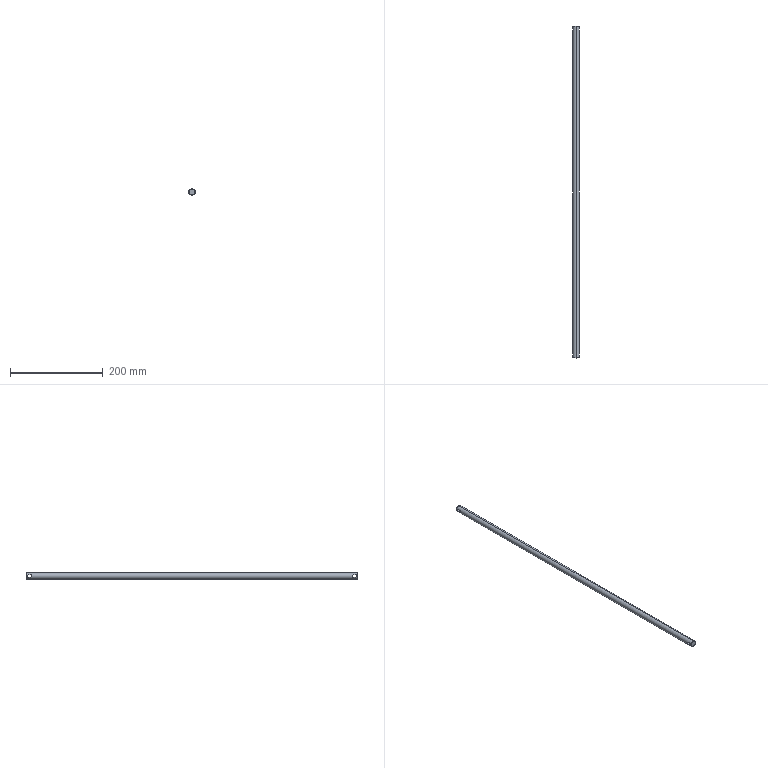Part | SolidWorks | features Chamfer 1, Extrusion 1, ICE 1 | 1 solid | 16 faces | box 14 x 715 x 14 mm | volume 108794 mm3 | cylinder 6 | plane 6 | cone 4 | commonest cylinder face diameters 6 x4 14 x2
STEP:
#1=CARTESIAN_POINT('',(0.,357.5,6.5));
#2=VERTEX_POINT('',#1);
#3=CARTESIAN_POINT('',(0.,357.5,-6.5));
#4=VERTEX_POINT('',#3);
#5=CARTESIAN_POINT('',(0.,357.5,0.));
#6=DIRECTION('',(0.,1.,0.));
#7=DIRECTION('',(0.,0.,1.));
#8=AXIS2_PLACEMENT_3D('',#5,#6,#7);
#9=CIRCLE('',#8,6.5);
#10=EDGE_CURVE('',#2,#4,#9,.T.);
#11=ORIENTED_EDGE('',*,*,#10,.F.);
#12=CARTESIAN_POINT('',(0.,357.,7.));
#13=VERTEX_POINT('',#12);
#14=CARTESIAN_POINT('',(0.,357.5,6.5));
#15=DIRECTION('',(0.,-0.7071,0.7071));
#16=VECTOR('',#15,1000.);
#17=LINE('',#14,#16);
#18=EDGE_CURVE('',#2,#13,#17,.T.);
#19=ORIENTED_EDGE('',*,*,#18,.T.);
#20=CARTESIAN_POINT('',(0.,357.,-7.));
#21=VERTEX_POINT('',#20);
#22=CARTESIAN_POINT('',(0.,357.,0.));
#23=DIRECTION('',(0.,-1.,0.));
#24=DIRECTION('',(0.,0.,1.));
#25=AXIS2_PLACEMENT_3D('',#22,#23,#24);
#26=CIRCLE('',#25,7.);
#27=EDGE_CURVE('',#21,#13,#26,.T.);
#28=ORIENTED_EDGE('',*,*,#27,.F.);
#29=CARTESIAN_POINT('',(0.,357.5,-6.5));
#30=DIRECTION('',(0.,-0.7071,-0.7071));
#31=VECTOR('',#30,1000.);
#32=LINE('',#29,#31);
#33=EDGE_CURVE('',#4,#21,#32,.T.);
#34=ORIENTED_EDGE('',*,*,#33,.F.);
#35=EDGE_LOOP('',(#11,#19,#28,#34));
#36=FACE_OUTER_BOUND('',#35,.T.);
#37=CARTESIAN_POINT('',(0.,357.5,0.));
#38=DIRECTION('',(0.,-1.,0.));
#39=DIRECTION('',(0.,0.,-1.));
#40=AXIS2_PLACEMENT_3D('',#37,#38,#39);
#41=CONICAL_SURFACE('',#40,6.5,0.7854);
#42=ADVANCED_FACE('',(#36),#41,.T.);
#43=CARTESIAN_POINT('',(0.,-357.5,-6.5));
#44=VERTEX_POINT('',#43);
#45=CARTESIAN_POINT('',(0.,-357.5,6.5));
#46=VERTEX_POINT('',#45);
#47=CARTESIAN_POINT('',(0.,-357.5,0.));
#48=DIRECTION('',(0.,-1.,0.));
#49=DIRECTION('',(0.,0.,1.));
#50=AXIS2_PLACEMENT_3D('',#47,#48,#49);
#51=CIRCLE('',#50,6.5);
#52=EDGE_CURVE('',#44,#46,#51,.T.);
#53=ORIENTED_EDGE('',*,*,#52,.F.);
#54=CARTESIAN_POINT('',(0.,-357.,-7.));
#55=VERTEX_POINT('',#54);
#56=CARTESIAN_POINT('',(0.,-357.,-7.));
#57=DIRECTION('',(0.,0.7071,-0.7071));
#58=VECTOR('',#57,1000.);
#59=LINE('',#56,#58);
#60=EDGE_CURVE('',#44,#55,#59,.T.);
#61=ORIENTED_EDGE('',*,*,#60,.T.);
#62=CARTESIAN_POINT('',(0.,-357.,7.));
#63=VERTEX_POINT('',#62);
#64=CARTESIAN_POINT('',(0.,-357.,0.));
#65=DIRECTION('',(0.,1.,0.));
#66=DIRECTION('',(0.,0.,1.));
#67=AXIS2_PLACEMENT_3D('',#64,#65,#66);
#68=CIRCLE('',#67,7.);
#69=EDGE_CURVE('',#63,#55,#68,.T.);
#70=ORIENTED_EDGE('',*,*,#69,.F.);
#71=CARTESIAN_POINT('',(0.,-357.,7.));
#72=DIRECTION('',(0.,0.7071,0.7071));
#73=VECTOR('',#72,1000.);
#74=LINE('',#71,#73);
#75=EDGE_CURVE('',#46,#63,#74,.T.);
#76=ORIENTED_EDGE('',*,*,#75,.F.);
#77=EDGE_LOOP('',(#53,#61,#70,#76));
#78=FACE_OUTER_BOUND('',#77,.T.);
#79=CARTESIAN_POINT('',(0.,-357.,0.));
#80=DIRECTION('',(0.,1.,0.));
#81=DIRECTION('',(0.,0.,1.));
#82=AXIS2_PLACEMENT_3D('',#79,#80,#81);
#83=CONICAL_SURFACE('',#82,7.,0.7854);
#84=ADVANCED_FACE('',(#78),#83,.T.);
#85=CARTESIAN_POINT('',(6.325,351.5,-3.));
#86=VERTEX_POINT('',#85);
#87=CARTESIAN_POINT('',(6.325,348.5,-3.));
#88=VERTEX_POINT('',#87);
#89=CARTESIAN_POINT('',(6.325,357.5,-3.));
#90=DIRECTION('',(0.,-1.,0.));
#91=VECTOR('',#90,1000.);
#92=LINE('',#89,#91);
#93=EDGE_CURVE('',#86,#88,#92,.T.);
#94=ORIENTED_EDGE('',*,*,#93,.T.);
#95=CARTESIAN_POINT('',(6.325,348.5,3.));
#96=VERTEX_POINT('',#95);
#97=CARTESIAN_POINT('',(6.325,348.5,-3.));
#98=CARTESIAN_POINT('',(6.325,348.299,-3.));
#99=CARTESIAN_POINT('',(6.334,348.102,-2.98));
#100=CARTESIAN_POINT('',(6.37,347.716,-2.902));
#101=CARTESIAN_POINT('',(6.397,347.524,-2.844));
#102=CARTESIAN_POINT('',(6.462,347.162,-2.692));
#103=CARTESIAN_POINT('',(6.5,346.991,-2.6));
#104=CARTESIAN_POINT('',(6.583,346.667,-2.383));
#105=CARTESIAN_POINT('',(6.627,346.515,-2.258));
#106=CARTESIAN_POINT('',(6.714,346.242,-1.985));
#107=CARTESIAN_POINT('',(6.757,346.118,-1.834));
#108=CARTESIAN_POINT('',(6.838,345.9,-1.509));
#109=CARTESIAN_POINT('',(6.873,345.808,-1.337));
#110=CARTESIAN_POINT('',(6.934,345.657,-0.977));
#111=CARTESIAN_POINT('',(6.959,345.598,-0.7853));
#112=CARTESIAN_POINT('',(6.991,345.52,-0.3967));
#113=CARTESIAN_POINT('',(7.,345.5,-0.2002));
#114=CARTESIAN_POINT('',(7.,345.5,0.197));
#115=CARTESIAN_POINT('',(6.991,345.52,0.3982));
#116=CARTESIAN_POINT('',(6.959,345.598,0.7855));
#117=CARTESIAN_POINT('',(6.934,345.656,0.9747));
#118=CARTESIAN_POINT('',(6.873,345.809,1.34));
#119=CARTESIAN_POINT('',(6.837,345.901,1.512));
#120=CARTESIAN_POINT('',(6.757,346.118,1.835));
#121=CARTESIAN_POINT('',(6.714,346.244,1.987));
#122=CARTESIAN_POINT('',(6.626,346.518,2.261));
#123=CARTESIAN_POINT('',(6.583,346.668,2.383));
#124=CARTESIAN_POINT('',(6.5,346.991,2.6));
#125=CARTESIAN_POINT('',(6.461,347.165,2.694));
#126=CARTESIAN_POINT('',(6.397,347.525,2.844));
#127=CARTESIAN_POINT('',(6.37,347.713,2.902));
#128=CARTESIAN_POINT('',(6.334,348.105,2.981));
#129=CARTESIAN_POINT('',(6.325,348.302,3.));
#130=CARTESIAN_POINT('',(6.325,348.5,3.));
#131=B_SPLINE_CURVE_WITH_KNOTS('',3,(#97,#98,#99,#100,#101,#102,#103,#104,#105,#106,#107,#108,#109,#110,#111,#112,#113,#114,#115,#116,#117,#118,#119,#120,#121,#122,#123,#124,#125,#126,#127,#128,#129,#130),.UNSPECIFIED.,.F.,.F.,(4,2,2,2,2,2,2,2,2,2,2,2,2,2,2,2,4),(0.,0.0005934,0.001187,0.00178,0.002374,0.002967,0.003561,0.004154,0.004748,0.005341,0.005934,0.006528,0.007121,0.007715,0.008308,0.008902,0.009495),.UNSPECIFIED.);
#132=EDGE_CURVE('',#88,#96,#131,.T.);
#133=ORIENTED_EDGE('',*,*,#132,.T.);
#134=CARTESIAN_POINT('',(6.325,351.5,3.));
#135=VERTEX_POINT('',#134);
#136=CARTESIAN_POINT('',(6.325,357.5,3.));
#137=DIRECTION('',(0.,1.,0.));
#138=VECTOR('',#137,1000.);
#139=LINE('',#136,#138);
#140=EDGE_CURVE('',#96,#135,#139,.T.);
#141=ORIENTED_EDGE('',*,*,#140,.T.);
#142=CARTESIAN_POINT('',(6.325,351.5,3.));
#143=CARTESIAN_POINT('',(6.325,351.698,3.));
#144=CARTESIAN_POINT('',(6.334,351.898,2.98));
#145=CARTESIAN_POINT('',(6.37,352.287,2.902));
#146=CARTESIAN_POINT('',(6.397,352.475,2.844));
#147=CARTESIAN_POINT('',(6.462,352.838,2.693));
#148=CARTESIAN_POINT('',(6.501,353.011,2.599));
#149=CARTESIAN_POINT('',(6.583,353.333,2.383));
#150=CARTESIAN_POINT('',(6.627,353.484,2.259));
#151=CARTESIAN_POINT('',(6.715,353.759,1.983));
#152=CARTESIAN_POINT('',(6.758,353.882,1.834));
#153=CARTESIAN_POINT('',(6.837,354.099,1.512));
#154=CARTESIAN_POINT('',(6.874,354.193,1.337));
#155=CARTESIAN_POINT('',(6.934,354.344,0.9749));
#156=CARTESIAN_POINT('',(6.958,354.402,0.7876));
#157=CARTESIAN_POINT('',(6.991,354.48,0.3996));
#158=CARTESIAN_POINT('',(7.,354.5,0.1985));
#159=CARTESIAN_POINT('',(7.,354.5,-0.1971));
#160=CARTESIAN_POINT('',(6.992,354.481,-0.3946));
#161=CARTESIAN_POINT('',(6.958,354.402,-0.7866));
#162=CARTESIAN_POINT('',(6.934,354.344,-0.9748));
#163=CARTESIAN_POINT('',(6.874,354.193,-1.337));
#164=CARTESIAN_POINT('',(6.837,354.099,-1.512));
#165=CARTESIAN_POINT('',(6.757,353.882,-1.835));
#166=CARTESIAN_POINT('',(6.714,353.759,-1.984));
#167=CARTESIAN_POINT('',(6.627,353.483,-2.26));
#168=CARTESIAN_POINT('',(6.583,353.332,-2.384));
#169=CARTESIAN_POINT('',(6.501,353.011,-2.599));
#170=CARTESIAN_POINT('',(6.462,352.838,-2.692));
#171=CARTESIAN_POINT('',(6.397,352.474,-2.844));
#172=CARTESIAN_POINT('',(6.37,352.286,-2.902));
#173=CARTESIAN_POINT('',(6.334,351.901,-2.98));
#174=CARTESIAN_POINT('',(6.325,351.701,-3.));
#175=CARTESIAN_POINT('',(6.325,351.5,-3.));
#176=B_SPLINE_CURVE_WITH_KNOTS('',3,(#142,#143,#144,#145,#146,#147,#148,#149,#150,#151,#152,#153,#154,#155,#156,#157,#158,#159,#160,#161,#162,#163,#164,#165,#166,#167,#168,#169,#170,#171,#172,#173,#174,#175),.UNSPECIFIED.,.F.,.F.,(4,2,2,2,2,2,2,2,2,2,2,2,2,2,2,2,4),(0.009495,0.01009,0.01068,0.01127,0.01187,0.01246,0.01305,0.01365,0.01424,0.01483,0.01542,0.01602,0.01661,0.0172,0.0178,0.01839,0.01898),.UNSPECIFIED.);
#177=EDGE_CURVE('',#135,#86,#176,.T.);
#178=ORIENTED_EDGE('',*,*,#177,.T.);
#179=EDGE_LOOP('',(#94,#133,#141,#178));
#180=FACE_BOUND('',#179,.T.);
#181=CARTESIAN_POINT('',(6.325,-351.5,3.));
#182=VERTEX_POINT('',#181);
#183=CARTESIAN_POINT('',(6.325,-348.5,3.));
#184=VERTEX_POINT('',#183);
#185=CARTESIAN_POINT('',(6.325,357.5,3.));
#186=DIRECTION('',(0.,1.,0.));
#187=VECTOR('',#186,1000.);
#188=LINE('',#185,#187);
#189=EDGE_CURVE('',#182,#184,#188,.T.);
#190=ORIENTED_EDGE('',*,*,#189,.T.);
#191=CARTESIAN_POINT('',(6.325,-348.5,-3.));
#192=VERTEX_POINT('',#191);
#193=CARTESIAN_POINT('',(6.325,-348.5,3.));
#194=CARTESIAN_POINT('',(6.325,-348.302,3.));
#195=CARTESIAN_POINT('',(6.334,-348.102,2.98));
#196=CARTESIAN_POINT('',(6.37,-347.713,2.902));
#197=CARTESIAN_POINT('',(6.397,-347.525,2.844));
#198=CARTESIAN_POINT('',(6.462,-347.162,2.693));
#199=CARTESIAN_POINT('',(6.501,-346.989,2.599));
#200=CARTESIAN_POINT('',(6.583,-346.667,2.383));
#201=CARTESIAN_POINT('',(6.627,-346.516,2.259));
#202=CARTESIAN_POINT('',(6.715,-346.241,1.983));
#203=CARTESIAN_POINT('',(6.758,-346.118,1.834));
#204=CARTESIAN_POINT('',(6.837,-345.901,1.512));
#205=CARTESIAN_POINT('',(6.874,-345.807,1.337));
#206=CARTESIAN_POINT('',(6.934,-345.656,0.9749));
#207=CARTESIAN_POINT('',(6.958,-345.598,0.7876));
#208=CARTESIAN_POINT('',(6.991,-345.52,0.3996));
#209=CARTESIAN_POINT('',(7.,-345.5,0.1985));
#210=CARTESIAN_POINT('',(7.,-345.5,-0.1971));
#211=CARTESIAN_POINT('',(6.992,-345.519,-0.3946));
#212=CARTESIAN_POINT('',(6.958,-345.598,-0.7866));
#213=CARTESIAN_POINT('',(6.934,-345.656,-0.9748));
#214=CARTESIAN_POINT('',(6.874,-345.807,-1.337));
#215=CARTESIAN_POINT('',(6.837,-345.901,-1.512));
#216=CARTESIAN_POINT('',(6.757,-346.118,-1.835));
#217=CARTESIAN_POINT('',(6.714,-346.241,-1.984));
#218=CARTESIAN_POINT('',(6.627,-346.517,-2.26));
#219=CARTESIAN_POINT('',(6.583,-346.668,-2.384));
#220=CARTESIAN_POINT('',(6.501,-346.989,-2.599));
#221=CARTESIAN_POINT('',(6.462,-347.162,-2.692));
#222=CARTESIAN_POINT('',(6.397,-347.526,-2.844));
#223=CARTESIAN_POINT('',(6.37,-347.714,-2.902));
#224=CARTESIAN_POINT('',(6.334,-348.099,-2.98));
#225=CARTESIAN_POINT('',(6.325,-348.299,-3.));
#226=CARTESIAN_POINT('',(6.325,-348.5,-3.));
#227=B_SPLINE_CURVE_WITH_KNOTS('',3,(#193,#194,#195,#196,#197,#198,#199,#200,#201,#202,#203,#204,#205,#206,#207,#208,#209,#210,#211,#212,#213,#214,#215,#216,#217,#218,#219,#220,#221,#222,#223,#224,#225,#226),.UNSPECIFIED.,.F.,.F.,(4,2,2,2,2,2,2,2,2,2,2,2,2,2,2,2,4),(0.009495,0.01009,0.01068,0.01127,0.01187,0.01246,0.01305,0.01365,0.01424,0.01483,0.01542,0.01602,0.01661,0.0172,0.0178,0.01839,0.01898),.UNSPECIFIED.);
#228=EDGE_CURVE('',#184,#192,#227,.T.);
#229=ORIENTED_EDGE('',*,*,#228,.T.);
#230=CARTESIAN_POINT('',(6.325,-351.5,-3.));
#231=VERTEX_POINT('',#230);
#232=CARTESIAN_POINT('',(6.325,357.5,-3.));
#233=DIRECTION('',(0.,-1.,0.));
#234=VECTOR('',#233,1000.);
#235=LINE('',#232,#234);
#236=EDGE_CURVE('',#192,#231,#235,.T.);
#237=ORIENTED_EDGE('',*,*,#236,.T.);
#238=CARTESIAN_POINT('',(6.325,-351.5,-3.));
#239=CARTESIAN_POINT('',(6.325,-351.701,-3.));
#240=CARTESIAN_POINT('',(6.334,-351.898,-2.98));
#241=CARTESIAN_POINT('',(6.37,-352.284,-2.902));
#242=CARTESIAN_POINT('',(6.397,-352.476,-2.844));
#243=CARTESIAN_POINT('',(6.462,-352.838,-2.692));
#244=CARTESIAN_POINT('',(6.5,-353.009,-2.6));
#245=CARTESIAN_POINT('',(6.583,-353.333,-2.383));
#246=CARTESIAN_POINT('',(6.627,-353.485,-2.258));
#247=CARTESIAN_POINT('',(6.714,-353.758,-1.985));
#248=CARTESIAN_POINT('',(6.757,-353.882,-1.834));
#249=CARTESIAN_POINT('',(6.838,-354.1,-1.509));
#250=CARTESIAN_POINT('',(6.873,-354.192,-1.337));
#251=CARTESIAN_POINT('',(6.934,-354.343,-0.977));
#252=CARTESIAN_POINT('',(6.959,-354.402,-0.7853));
#253=CARTESIAN_POINT('',(6.991,-354.48,-0.3967));
#254=CARTESIAN_POINT('',(7.,-354.5,-0.2002));
#255=CARTESIAN_POINT('',(7.,-354.5,0.197));
#256=CARTESIAN_POINT('',(6.991,-354.48,0.3982));
#257=CARTESIAN_POINT('',(6.959,-354.402,0.7855));
#258=CARTESIAN_POINT('',(6.934,-354.344,0.9747));
#259=CARTESIAN_POINT('',(6.873,-354.191,1.34));
#260=CARTESIAN_POINT('',(6.837,-354.099,1.512));
#261=CARTESIAN_POINT('',(6.757,-353.882,1.835));
#262=CARTESIAN_POINT('',(6.714,-353.756,1.987));
#263=CARTESIAN_POINT('',(6.626,-353.482,2.261));
#264=CARTESIAN_POINT('',(6.583,-353.332,2.383));
#265=CARTESIAN_POINT('',(6.5,-353.009,2.6));
#266=CARTESIAN_POINT('',(6.461,-352.835,2.694));
#267=CARTESIAN_POINT('',(6.397,-352.475,2.844));
#268=CARTESIAN_POINT('',(6.37,-352.287,2.902));
#269=CARTESIAN_POINT('',(6.334,-351.895,2.981));
#270=CARTESIAN_POINT('',(6.325,-351.698,3.));
#271=CARTESIAN_POINT('',(6.325,-351.5,3.));
#272=B_SPLINE_CURVE_WITH_KNOTS('',3,(#238,#239,#240,#241,#242,#243,#244,#245,#246,#247,#248,#249,#250,#251,#252,#253,#254,#255,#256,#257,#258,#259,#260,#261,#262,#263,#264,#265,#266,#267,#268,#269,#270,#271),.UNSPECIFIED.,.F.,.F.,(4,2,2,2,2,2,2,2,2,2,2,2,2,2,2,2,4),(0.,0.0005934,0.001187,0.00178,0.002374,0.002967,0.003561,0.004154,0.004748,0.005341,0.005934,0.006528,0.007121,0.007715,0.008308,0.008902,0.009495),.UNSPECIFIED.);
#273=EDGE_CURVE('',#231,#182,#272,.T.);
#274=ORIENTED_EDGE('',*,*,#273,.T.);
#275=EDGE_LOOP('',(#190,#229,#237,#274));
#276=FACE_BOUND('',#275,.T.);
#277=ORIENTED_EDGE('',*,*,#27,.T.);
#278=CARTESIAN_POINT('',(0.,357.5,7.));
#279=DIRECTION('',(0.,-1.,0.));
#280=VECTOR('',#279,1000.);
#281=LINE('',#278,#280);
#282=EDGE_CURVE('',#13,#63,#281,.T.);
#283=ORIENTED_EDGE('',*,*,#282,.T.);
#284=ORIENTED_EDGE('',*,*,#69,.T.);
#285=CARTESIAN_POINT('',(0.,357.5,-7.));
#286=DIRECTION('',(0.,-1.,0.));
#287=VECTOR('',#286,1000.);
#288=LINE('',#285,#287);
#289=EDGE_CURVE('',#21,#55,#288,.T.);
#290=ORIENTED_EDGE('',*,*,#289,.F.);
#291=EDGE_LOOP('',(#277,#283,#284,#290));
#292=FACE_OUTER_BOUND('',#291,.T.);
#293=CARTESIAN_POINT('',(0.,357.5,0.));
#294=DIRECTION('',(0.,-1.,0.));
#295=DIRECTION('',(0.,0.,-1.));
#296=AXIS2_PLACEMENT_3D('',#293,#294,#295);
#297=CYLINDRICAL_SURFACE('',#296,7.);
#298=ADVANCED_FACE('',(#180,#276,#292),#297,.T.);
#299=ORIENTED_EDGE('',*,*,#282,.F.);
#300=CARTESIAN_POINT('',(0.,357.,0.));
#301=DIRECTION('',(0.,-1.,0.));
#302=DIRECTION('',(0.,0.,1.));
#303=AXIS2_PLACEMENT_3D('',#300,#301,#302);
#304=CIRCLE('',#303,7.);
#305=EDGE_CURVE('',#13,#21,#304,.T.);
#306=ORIENTED_EDGE('',*,*,#305,.T.);
#307=ORIENTED_EDGE('',*,*,#289,.T.);
#308=CARTESIAN_POINT('',(0.,-357.,0.));
#309=DIRECTION('',(0.,1.,0.));
#310=DIRECTION('',(0.,0.,1.));
#311=AXIS2_PLACEMENT_3D('',#308,#309,#310);
#312=CIRCLE('',#311,7.);
#313=EDGE_CURVE('',#55,#63,#312,.T.);
#314=ORIENTED_EDGE('',*,*,#313,.T.);
#315=EDGE_LOOP('',(#299,#306,#307,#314));
#316=FACE_OUTER_BOUND('',#315,.T.);
#317=CARTESIAN_POINT('',(-6.325,-351.5,-3.));
#318=VERTEX_POINT('',#317);
#319=CARTESIAN_POINT('',(-6.325,-348.5,-3.));
#320=VERTEX_POINT('',#319);
#321=CARTESIAN_POINT('',(-6.325,357.5,-3.));
#322=DIRECTION('',(0.,1.,0.));
#323=VECTOR('',#322,1000.);
#324=LINE('',#321,#323);
#325=EDGE_CURVE('',#318,#320,#324,.T.);
#326=ORIENTED_EDGE('',*,*,#325,.T.);
#327=CARTESIAN_POINT('',(-6.325,-348.5,3.));
#328=VERTEX_POINT('',#327);
#329=CARTESIAN_POINT('',(-6.325,-348.5,-3.));
#330=CARTESIAN_POINT('',(-6.325,-348.299,-3.));
#331=CARTESIAN_POINT('',(-6.334,-348.102,-2.98));
#332=CARTESIAN_POINT('',(-6.37,-347.716,-2.902));
#333=CARTESIAN_POINT('',(-6.397,-347.524,-2.844));
#334=CARTESIAN_POINT('',(-6.462,-347.162,-2.692));
#335=CARTESIAN_POINT('',(-6.5,-346.991,-2.6));
#336=CARTESIAN_POINT('',(-6.583,-346.667,-2.383));
#337=CARTESIAN_POINT('',(-6.627,-346.515,-2.258));
#338=CARTESIAN_POINT('',(-6.714,-346.242,-1.985));
#339=CARTESIAN_POINT('',(-6.757,-346.118,-1.834));
#340=CARTESIAN_POINT('',(-6.838,-345.9,-1.509));
#341=CARTESIAN_POINT('',(-6.873,-345.808,-1.337));
#342=CARTESIAN_POINT('',(-6.934,-345.657,-0.977));
#343=CARTESIAN_POINT('',(-6.959,-345.598,-0.7853));
#344=CARTESIAN_POINT('',(-6.991,-345.52,-0.3967));
#345=CARTESIAN_POINT('',(-7.,-345.5,-0.2002));
#346=CARTESIAN_POINT('',(-7.,-345.5,0.197));
#347=CARTESIAN_POINT('',(-6.991,-345.52,0.3982));
#348=CARTESIAN_POINT('',(-6.959,-345.598,0.7855));
#349=CARTESIAN_POINT('',(-6.934,-345.656,0.9747));
#350=CARTESIAN_POINT('',(-6.873,-345.809,1.34));
#351=CARTESIAN_POINT('',(-6.837,-345.901,1.512));
#352=CARTESIAN_POINT('',(-6.757,-346.118,1.835));
#353=CARTESIAN_POINT('',(-6.714,-346.244,1.987));
#354=CARTESIAN_POINT('',(-6.626,-346.518,2.261));
#355=CARTESIAN_POINT('',(-6.583,-346.668,2.383));
#356=CARTESIAN_POINT('',(-6.5,-346.991,2.6));
#357=CARTESIAN_POINT('',(-6.461,-347.165,2.694));
#358=CARTESIAN_POINT('',(-6.397,-347.525,2.844));
#359=CARTESIAN_POINT('',(-6.37,-347.713,2.902));
#360=CARTESIAN_POINT('',(-6.334,-348.105,2.981));
#361=CARTESIAN_POINT('',(-6.325,-348.302,3.));
#362=CARTESIAN_POINT('',(-6.325,-348.5,3.));
#363=B_SPLINE_CURVE_WITH_KNOTS('',3,(#329,#330,#331,#332,#333,#334,#335,#336,#337,#338,#339,#340,#341,#342,#343,#344,#345,#346,#347,#348,#349,#350,#351,#352,#353,#354,#355,#356,#357,#358,#359,#360,#361,#362),.UNSPECIFIED.,.F.,.F.,(4,2,2,2,2,2,2,2,2,2,2,2,2,2,2,2,4),(0.,0.0005934,0.001187,0.00178,0.002374,0.002967,0.003561,0.004154,0.004748,0.005341,0.005934,0.006528,0.007121,0.007715,0.008308,0.008902,0.009495),.UNSPECIFIED.);
#364=EDGE_CURVE('',#320,#328,#363,.T.);
#365=ORIENTED_EDGE('',*,*,#364,.T.);
#366=CARTESIAN_POINT('',(-6.325,-351.5,3.));
#367=VERTEX_POINT('',#366);
#368=CARTESIAN_POINT('',(-6.325,357.5,3.));
#369=DIRECTION('',(0.,-1.,0.));
#370=VECTOR('',#369,1000.);
#371=LINE('',#368,#370);
#372=EDGE_CURVE('',#328,#367,#371,.T.);
#373=ORIENTED_EDGE('',*,*,#372,.T.);
#374=CARTESIAN_POINT('',(-6.325,-351.5,3.));
#375=CARTESIAN_POINT('',(-6.325,-351.698,3.));
#376=CARTESIAN_POINT('',(-6.334,-351.898,2.98));
#377=CARTESIAN_POINT('',(-6.37,-352.287,2.902));
#378=CARTESIAN_POINT('',(-6.397,-352.475,2.844));
#379=CARTESIAN_POINT('',(-6.462,-352.838,2.693));
#380=CARTESIAN_POINT('',(-6.501,-353.011,2.599));
#381=CARTESIAN_POINT('',(-6.583,-353.333,2.383));
#382=CARTESIAN_POINT('',(-6.627,-353.484,2.259));
#383=CARTESIAN_POINT('',(-6.715,-353.759,1.983));
#384=CARTESIAN_POINT('',(-6.758,-353.882,1.834));
#385=CARTESIAN_POINT('',(-6.837,-354.099,1.512));
#386=CARTESIAN_POINT('',(-6.874,-354.193,1.337));
#387=CARTESIAN_POINT('',(-6.934,-354.344,0.9749));
#388=CARTESIAN_POINT('',(-6.958,-354.402,0.7876));
#389=CARTESIAN_POINT('',(-6.991,-354.48,0.3996));
#390=CARTESIAN_POINT('',(-7.,-354.5,0.1985));
#391=CARTESIAN_POINT('',(-7.,-354.5,-0.1971));
#392=CARTESIAN_POINT('',(-6.992,-354.481,-0.3946));
#393=CARTESIAN_POINT('',(-6.958,-354.402,-0.7866));
#394=CARTESIAN_POINT('',(-6.934,-354.344,-0.9748));
#395=CARTESIAN_POINT('',(-6.874,-354.193,-1.337));
#396=CARTESIAN_POINT('',(-6.837,-354.099,-1.512));
#397=CARTESIAN_POINT('',(-6.757,-353.882,-1.835));
#398=CARTESIAN_POINT('',(-6.714,-353.759,-1.984));
#399=CARTESIAN_POINT('',(-6.627,-353.483,-2.26));
#400=CARTESIAN_POINT('',(-6.583,-353.332,-2.384));
#401=CARTESIAN_POINT('',(-6.501,-353.011,-2.599));
#402=CARTESIAN_POINT('',(-6.462,-352.838,-2.692));
#403=CARTESIAN_POINT('',(-6.397,-352.474,-2.844));
#404=CARTESIAN_POINT('',(-6.37,-352.286,-2.902));
#405=CARTESIAN_POINT('',(-6.334,-351.901,-2.98));
#406=CARTESIAN_POINT('',(-6.325,-351.701,-3.));
#407=CARTESIAN_POINT('',(-6.325,-351.5,-3.));
#408=B_SPLINE_CURVE_WITH_KNOTS('',3,(#374,#375,#376,#377,#378,#379,#380,#381,#382,#383,#384,#385,#386,#387,#388,#389,#390,#391,#392,#393,#394,#395,#396,#397,#398,#399,#400,#401,#402,#403,#404,#405,#406,#407),.UNSPECIFIED.,.F.,.F.,(4,2,2,2,2,2,2,2,2,2,2,2,2,2,2,2,4),(0.009495,0.01009,0.01068,0.01127,0.01187,0.01246,0.01305,0.01365,0.01424,0.01483,0.01542,0.01602,0.01661,0.0172,0.0178,0.01839,0.01898),.UNSPECIFIED.);
#409=EDGE_CURVE('',#367,#318,#408,.T.);
#410=ORIENTED_EDGE('',*,*,#409,.T.);
#411=EDGE_LOOP('',(#326,#365,#373,#410));
#412=FACE_BOUND('',#411,.T.);
#413=CARTESIAN_POINT('',(-6.325,351.5,3.));
#414=VERTEX_POINT('',#413);
#415=CARTESIAN_POINT('',(-6.325,348.5,3.));
#416=VERTEX_POINT('',#415);
#417=CARTESIAN_POINT('',(-6.325,357.5,3.));
#418=DIRECTION('',(0.,-1.,0.));
#419=VECTOR('',#418,1000.);
#420=LINE('',#417,#419);
#421=EDGE_CURVE('',#414,#416,#420,.T.);
#422=ORIENTED_EDGE('',*,*,#421,.T.);
#423=CARTESIAN_POINT('',(-6.325,348.5,-3.));
#424=VERTEX_POINT('',#423);
#425=CARTESIAN_POINT('',(-6.325,348.5,3.));
#426=CARTESIAN_POINT('',(-6.325,348.302,3.));
#427=CARTESIAN_POINT('',(-6.334,348.102,2.98));
#428=CARTESIAN_POINT('',(-6.37,347.713,2.902));
#429=CARTESIAN_POINT('',(-6.397,347.525,2.844));
#430=CARTESIAN_POINT('',(-6.462,347.162,2.693));
#431=CARTESIAN_POINT('',(-6.501,346.989,2.599));
#432=CARTESIAN_POINT('',(-6.583,346.667,2.383));
#433=CARTESIAN_POINT('',(-6.627,346.516,2.259));
#434=CARTESIAN_POINT('',(-6.715,346.241,1.983));
#435=CARTESIAN_POINT('',(-6.758,346.118,1.834));
#436=CARTESIAN_POINT('',(-6.837,345.901,1.512));
#437=CARTESIAN_POINT('',(-6.874,345.807,1.337));
#438=CARTESIAN_POINT('',(-6.934,345.656,0.9749));
#439=CARTESIAN_POINT('',(-6.958,345.598,0.7876));
#440=CARTESIAN_POINT('',(-6.991,345.52,0.3996));
#441=CARTESIAN_POINT('',(-7.,345.5,0.1985));
#442=CARTESIAN_POINT('',(-7.,345.5,-0.1971));
#443=CARTESIAN_POINT('',(-6.992,345.519,-0.3946));
#444=CARTESIAN_POINT('',(-6.958,345.598,-0.7866));
#445=CARTESIAN_POINT('',(-6.934,345.656,-0.9748));
#446=CARTESIAN_POINT('',(-6.874,345.807,-1.337));
#447=CARTESIAN_POINT('',(-6.837,345.901,-1.512));
#448=CARTESIAN_POINT('',(-6.757,346.118,-1.835));
#449=CARTESIAN_POINT('',(-6.714,346.241,-1.984));
#450=CARTESIAN_POINT('',(-6.627,346.517,-2.26));
#451=CARTESIAN_POINT('',(-6.583,346.668,-2.384));
#452=CARTESIAN_POINT('',(-6.501,346.989,-2.599));
#453=CARTESIAN_POINT('',(-6.462,347.162,-2.692));
#454=CARTESIAN_POINT('',(-6.397,347.526,-2.844));
#455=CARTESIAN_POINT('',(-6.37,347.714,-2.902));
#456=CARTESIAN_POINT('',(-6.334,348.099,-2.98));
#457=CARTESIAN_POINT('',(-6.325,348.299,-3.));
#458=CARTESIAN_POINT('',(-6.325,348.5,-3.));
#459=B_SPLINE_CURVE_WITH_KNOTS('',3,(#425,#426,#427,#428,#429,#430,#431,#432,#433,#434,#435,#436,#437,#438,#439,#440,#441,#442,#443,#444,#445,#446,#447,#448,#449,#450,#451,#452,#453,#454,#455,#456,#457,#458),.UNSPECIFIED.,.F.,.F.,(4,2,2,2,2,2,2,2,2,2,2,2,2,2,2,2,4),(0.009495,0.01009,0.01068,0.01127,0.01187,0.01246,0.01305,0.01365,0.01424,0.01483,0.01542,0.01602,0.01661,0.0172,0.0178,0.01839,0.01898),.UNSPECIFIED.);
#460=EDGE_CURVE('',#416,#424,#459,.T.);
#461=ORIENTED_EDGE('',*,*,#460,.T.);
#462=CARTESIAN_POINT('',(-6.325,351.5,-3.));
#463=VERTEX_POINT('',#462);
#464=CARTESIAN_POINT('',(-6.325,357.5,-3.));
#465=DIRECTION('',(0.,1.,0.));
#466=VECTOR('',#465,1000.);
#467=LINE('',#464,#466);
#468=EDGE_CURVE('',#424,#463,#467,.T.);
#469=ORIENTED_EDGE('',*,*,#468,.T.);
#470=CARTESIAN_POINT('',(-6.325,351.5,-3.));
#471=CARTESIAN_POINT('',(-6.325,351.701,-3.));
#472=CARTESIAN_POINT('',(-6.334,351.898,-2.98));
#473=CARTESIAN_POINT('',(-6.37,352.284,-2.902));
#474=CARTESIAN_POINT('',(-6.397,352.476,-2.844));
#475=CARTESIAN_POINT('',(-6.462,352.838,-2.692));
#476=CARTESIAN_POINT('',(-6.5,353.009,-2.6));
#477=CARTESIAN_POINT('',(-6.583,353.333,-2.383));
#478=CARTESIAN_POINT('',(-6.627,353.485,-2.258));
#479=CARTESIAN_POINT('',(-6.714,353.758,-1.985));
#480=CARTESIAN_POINT('',(-6.757,353.882,-1.834));
#481=CARTESIAN_POINT('',(-6.838,354.1,-1.509));
#482=CARTESIAN_POINT('',(-6.873,354.192,-1.337));
#483=CARTESIAN_POINT('',(-6.934,354.343,-0.977));
#484=CARTESIAN_POINT('',(-6.959,354.402,-0.7853));
#485=CARTESIAN_POINT('',(-6.991,354.48,-0.3967));
#486=CARTESIAN_POINT('',(-7.,354.5,-0.2002));
#487=CARTESIAN_POINT('',(-7.,354.5,0.197));
#488=CARTESIAN_POINT('',(-6.991,354.48,0.3982));
#489=CARTESIAN_POINT('',(-6.959,354.402,0.7855));
#490=CARTESIAN_POINT('',(-6.934,354.344,0.9747));
#491=CARTESIAN_POINT('',(-6.873,354.191,1.34));
#492=CARTESIAN_POINT('',(-6.837,354.099,1.512));
#493=CARTESIAN_POINT('',(-6.757,353.882,1.835));
#494=CARTESIAN_POINT('',(-6.714,353.756,1.987));
#495=CARTESIAN_POINT('',(-6.626,353.482,2.261));
#496=CARTESIAN_POINT('',(-6.583,353.332,2.383));
#497=CARTESIAN_POINT('',(-6.5,353.009,2.6));
#498=CARTESIAN_POINT('',(-6.461,352.835,2.694));
#499=CARTESIAN_POINT('',(-6.397,352.475,2.844));
#500=CARTESIAN_POINT('',(-6.37,352.287,2.902));
#501=CARTESIAN_POINT('',(-6.334,351.895,2.981));
#502=CARTESIAN_POINT('',(-6.325,351.698,3.));
#503=CARTESIAN_POINT('',(-6.325,351.5,3.));
#504=B_SPLINE_CURVE_WITH_KNOTS('',3,(#470,#471,#472,#473,#474,#475,#476,#477,#478,#479,#480,#481,#482,#483,#484,#485,#486,#487,#488,#489,#490,#491,#492,#493,#494,#495,#496,#497,#498,#499,#500,#501,#502,#503),.UNSPECIFIED.,.F.,.F.,(4,2,2,2,2,2,2,2,2,2,2,2,2,2,2,2,4),(0.,0.0005934,0.001187,0.00178,0.002374,0.002967,0.003561,0.004154,0.004748,0.005341,0.005934,0.006528,0.007121,0.007715,0.008308,0.008902,0.009495),.UNSPECIFIED.);
#505=EDGE_CURVE('',#463,#414,#504,.T.);
#506=ORIENTED_EDGE('',*,*,#505,.T.);
#507=EDGE_LOOP('',(#422,#461,#469,#506));
#508=FACE_BOUND('',#507,.T.);
#509=CARTESIAN_POINT('',(0.,357.5,0.));
#510=DIRECTION('',(0.,-1.,0.));
#511=DIRECTION('',(0.,0.,-1.));
#512=AXIS2_PLACEMENT_3D('',#509,#510,#511);
#513=CYLINDRICAL_SURFACE('',#512,7.);
#514=ADVANCED_FACE('',(#316,#412,#508),#513,.T.);
#515=CARTESIAN_POINT('',(0.,357.5,0.));
#516=DIRECTION('',(0.,1.,0.));
#517=DIRECTION('',(0.,0.,1.));
#518=AXIS2_PLACEMENT_3D('',#515,#516,#517);
#519=CIRCLE('',#518,6.5);
#520=EDGE_CURVE('',#4,#2,#519,.T.);
#521=ORIENTED_EDGE('',*,*,#520,.T.);
#522=ORIENTED_EDGE('',*,*,#10,.T.);
#523=EDGE_LOOP('',(#521,#522));
#524=FACE_OUTER_BOUND('',#523,.T.);
#525=CARTESIAN_POINT('',(0.,357.5,0.));
#526=DIRECTION('',(0.,1.,0.));
#527=DIRECTION('',(0.,0.,1.));
#528=AXIS2_PLACEMENT_3D('',#525,#526,#527);
#529=PLANE('',#528);
#530=ADVANCED_FACE('',(#524),#529,.T.);
#531=CARTESIAN_POINT('',(0.,-357.5,0.));
#532=DIRECTION('',(0.,-1.,0.));
#533=DIRECTION('',(0.,0.,1.));
#534=AXIS2_PLACEMENT_3D('',#531,#532,#533);
#535=CIRCLE('',#534,6.5);
#536=EDGE_CURVE('',#46,#44,#535,.T.);
#537=ORIENTED_EDGE('',*,*,#536,.T.);
#538=ORIENTED_EDGE('',*,*,#52,.T.);
#539=EDGE_LOOP('',(#537,#538));
#540=FACE_OUTER_BOUND('',#539,.T.);
#541=CARTESIAN_POINT('',(0.,-357.5,0.));
#542=DIRECTION('',(0.,1.,0.));
#543=DIRECTION('',(0.,0.,1.));
#544=AXIS2_PLACEMENT_3D('',#541,#542,#543);
#545=PLANE('',#544);
#546=ADVANCED_FACE('',(#540),#545,.F.);
#547=ORIENTED_EDGE('',*,*,#60,.F.);
#548=ORIENTED_EDGE('',*,*,#536,.F.);
#549=ORIENTED_EDGE('',*,*,#75,.T.);
#550=ORIENTED_EDGE('',*,*,#313,.F.);
#551=EDGE_LOOP('',(#547,#548,#549,#550));
#552=FACE_OUTER_BOUND('',#551,.T.);
#553=CARTESIAN_POINT('',(0.,-357.,0.));
#554=DIRECTION('',(0.,1.,0.));
#555=DIRECTION('',(0.,0.,1.));
#556=AXIS2_PLACEMENT_3D('',#553,#554,#555);
#557=CONICAL_SURFACE('',#556,7.,0.7854);
#558=ADVANCED_FACE('',(#552),#557,.T.);
#559=ORIENTED_EDGE('',*,*,#18,.F.);
#560=ORIENTED_EDGE('',*,*,#520,.F.);
#561=ORIENTED_EDGE('',*,*,#33,.T.);
#562=ORIENTED_EDGE('',*,*,#305,.F.);
#563=EDGE_LOOP('',(#559,#560,#561,#562));
#564=FACE_OUTER_BOUND('',#563,.T.);
#565=CARTESIAN_POINT('',(0.,357.5,0.));
#566=DIRECTION('',(0.,-1.,0.));
#567=DIRECTION('',(0.,0.,-1.));
#568=AXIS2_PLACEMENT_3D('',#565,#566,#567);
#569=CONICAL_SURFACE('',#568,6.5,0.7854);
#570=ADVANCED_FACE('',(#564),#569,.T.);
#571=CARTESIAN_POINT('',(-7.,351.5,-3.));
#572=DIRECTION('',(1.,0.,0.));
#573=VECTOR('',#572,1000.);
#574=LINE('',#571,#573);
#575=EDGE_CURVE('',#463,#86,#574,.T.);
#576=ORIENTED_EDGE('',*,*,#575,.T.);
#577=ORIENTED_EDGE('',*,*,#177,.F.);
#578=CARTESIAN_POINT('',(-7.,351.5,3.));
#579=DIRECTION('',(1.,0.,0.));
#580=VECTOR('',#579,1000.);
#581=LINE('',#578,#580);
#582=EDGE_CURVE('',#414,#135,#581,.T.);
#583=ORIENTED_EDGE('',*,*,#582,.F.);
#584=ORIENTED_EDGE('',*,*,#505,.F.);
#585=EDGE_LOOP('',(#576,#577,#583,#584));
#586=FACE_OUTER_BOUND('',#585,.T.);
#587=CARTESIAN_POINT('',(-7.,351.5,0.));
#588=DIRECTION('',(1.,0.,0.));
#589=DIRECTION('',(0.,0.,-1.));
#590=AXIS2_PLACEMENT_3D('',#587,#588,#589);
#591=CYLINDRICAL_SURFACE('',#590,3.);
#592=ADVANCED_FACE('',(#586),#591,.F.);
#593=ORIENTED_EDGE('',*,*,#575,.F.);
#594=ORIENTED_EDGE('',*,*,#468,.F.);
#595=CARTESIAN_POINT('',(-7.,348.5,-3.));
#596=DIRECTION('',(1.,0.,0.));
#597=VECTOR('',#596,1000.);
#598=LINE('',#595,#597);
#599=EDGE_CURVE('',#424,#88,#598,.T.);
#600=ORIENTED_EDGE('',*,*,#599,.T.);
#601=ORIENTED_EDGE('',*,*,#93,.F.);
#602=EDGE_LOOP('',(#593,#594,#600,#601));
#603=FACE_OUTER_BOUND('',#602,.T.);
#604=CARTESIAN_POINT('',(-7.,351.5,-3.));
#605=DIRECTION('',(0.,0.,-1.));
#606=DIRECTION('',(0.,1.,0.));
#607=AXIS2_PLACEMENT_3D('',#604,#605,#606);
#608=PLANE('',#607);
#609=ADVANCED_FACE('',(#603),#608,.F.);
#610=CARTESIAN_POINT('',(-7.,348.5,3.));
#611=DIRECTION('',(1.,0.,0.));
#612=VECTOR('',#611,1000.);
#613=LINE('',#610,#612);
#614=EDGE_CURVE('',#416,#96,#613,.T.);
#615=ORIENTED_EDGE('',*,*,#614,.T.);
#616=ORIENTED_EDGE('',*,*,#132,.F.);
#617=ORIENTED_EDGE('',*,*,#599,.F.);
#618=ORIENTED_EDGE('',*,*,#460,.F.);
#619=EDGE_LOOP('',(#615,#616,#617,#618));
#620=FACE_OUTER_BOUND('',#619,.T.);
#621=CARTESIAN_POINT('',(-7.,348.5,0.));
#622=DIRECTION('',(1.,0.,0.));
#623=DIRECTION('',(0.,0.,-1.));
#624=AXIS2_PLACEMENT_3D('',#621,#622,#623);
#625=CYLINDRICAL_SURFACE('',#624,3.);
#626=ADVANCED_FACE('',(#620),#625,.F.);
#627=ORIENTED_EDGE('',*,*,#582,.T.);
#628=ORIENTED_EDGE('',*,*,#140,.F.);
#629=ORIENTED_EDGE('',*,*,#614,.F.);
#630=ORIENTED_EDGE('',*,*,#421,.F.);
#631=EDGE_LOOP('',(#627,#628,#629,#630));
#632=FACE_OUTER_BOUND('',#631,.T.);
#633=CARTESIAN_POINT('',(-7.,351.5,3.));
#634=DIRECTION('',(0.,0.,1.));
#635=DIRECTION('',(0.,-1.,0.));
#636=AXIS2_PLACEMENT_3D('',#633,#634,#635);
#637=PLANE('',#636);
#638=ADVANCED_FACE('',(#632),#637,.F.);
#639=CARTESIAN_POINT('',(-7.,-351.5,3.));
#640=DIRECTION('',(1.,0.,0.));
#641=VECTOR('',#640,1000.);
#642=LINE('',#639,#641);
#643=EDGE_CURVE('',#367,#182,#642,.T.);
#644=ORIENTED_EDGE('',*,*,#643,.T.);
#645=ORIENTED_EDGE('',*,*,#273,.F.);
#646=CARTESIAN_POINT('',(-7.,-351.5,-3.));
#647=DIRECTION('',(1.,0.,0.));
#648=VECTOR('',#647,1000.);
#649=LINE('',#646,#648);
#650=EDGE_CURVE('',#318,#231,#649,.T.);
#651=ORIENTED_EDGE('',*,*,#650,.F.);
#652=ORIENTED_EDGE('',*,*,#409,.F.);
#653=EDGE_LOOP('',(#644,#645,#651,#652));
#654=FACE_OUTER_BOUND('',#653,.T.);
#655=CARTESIAN_POINT('',(-7.,-351.5,0.));
#656=DIRECTION('',(1.,0.,0.));
#657=DIRECTION('',(0.,0.,-1.));
#658=AXIS2_PLACEMENT_3D('',#655,#656,#657);
#659=CYLINDRICAL_SURFACE('',#658,3.);
#660=ADVANCED_FACE('',(#654),#659,.F.);
#661=CARTESIAN_POINT('',(-7.,-348.5,3.));
#662=DIRECTION('',(1.,0.,0.));
#663=VECTOR('',#662,1000.);
#664=LINE('',#661,#663);
#665=EDGE_CURVE('',#328,#184,#664,.T.);
#666=ORIENTED_EDGE('',*,*,#665,.T.);
#667=ORIENTED_EDGE('',*,*,#189,.F.);
#668=ORIENTED_EDGE('',*,*,#643,.F.);
#669=ORIENTED_EDGE('',*,*,#372,.F.);
#670=EDGE_LOOP('',(#666,#667,#668,#669));
#671=FACE_OUTER_BOUND('',#670,.T.);
#672=CARTESIAN_POINT('',(-7.,-351.5,3.));
#673=DIRECTION('',(0.,0.,1.));
#674=DIRECTION('',(0.,-1.,0.));
#675=AXIS2_PLACEMENT_3D('',#672,#673,#674);
#676=PLANE('',#675);
#677=ADVANCED_FACE('',(#671),#676,.F.);
#678=CARTESIAN_POINT('',(-7.,-348.5,-3.));
#679=DIRECTION('',(1.,0.,0.));
#680=VECTOR('',#679,1000.);
#681=LINE('',#678,#680);
#682=EDGE_CURVE('',#320,#192,#681,.T.);
#683=ORIENTED_EDGE('',*,*,#682,.T.);
#684=ORIENTED_EDGE('',*,*,#228,.F.);
#685=ORIENTED_EDGE('',*,*,#665,.F.);
#686=ORIENTED_EDGE('',*,*,#364,.F.);
#687=EDGE_LOOP('',(#683,#684,#685,#686));
#688=FACE_OUTER_BOUND('',#687,.T.);
#689=CARTESIAN_POINT('',(-7.,-348.5,0.));
#690=DIRECTION('',(1.,0.,0.));
#691=DIRECTION('',(0.,0.,-1.));
#692=AXIS2_PLACEMENT_3D('',#689,#690,#691);
#693=CYLINDRICAL_SURFACE('',#692,3.);
#694=ADVANCED_FACE('',(#688),#693,.F.);
#695=ORIENTED_EDGE('',*,*,#682,.F.);
#696=ORIENTED_EDGE('',*,*,#325,.F.);
#697=ORIENTED_EDGE('',*,*,#650,.T.);
#698=ORIENTED_EDGE('',*,*,#236,.F.);
#699=EDGE_LOOP('',(#695,#696,#697,#698));
#700=FACE_OUTER_BOUND('',#699,.T.);
#701=CARTESIAN_POINT('',(-7.,-351.5,-3.));
#702=DIRECTION('',(0.,0.,-1.));
#703=DIRECTION('',(0.,1.,0.));
#704=AXIS2_PLACEMENT_3D('',#701,#702,#703);
#705=PLANE('',#704);
#706=ADVANCED_FACE('',(#700),#705,.F.);
#707=CLOSED_SHELL('',(#42,#84,#298,#514,#530,#546,#558,#570,#592,#609,#626,#638,#660,#677,#694,#706));
#708=MANIFOLD_SOLID_BREP('',#707);
#709=CARTESIAN_POINT('',(0.,0.,0.));
#710=DIRECTION('',(0.,0.,1.));
#711=DIRECTION('',(1.,0.,0.));
#712=AXIS2_PLACEMENT_3D('',#709,#710,#711);
#713=(LENGTH_UNIT()NAMED_UNIT(*)SI_UNIT(.MILLI.,.METRE.));
#714=UNCERTAINTY_MEASURE_WITH_UNIT(LENGTH_MEASURE(0.00001),#713,'','');
#715=(NAMED_UNIT(*)PLANE_ANGLE_UNIT()SI_UNIT($,.RADIAN.));
#716=(NAMED_UNIT(*)SI_UNIT($,.STERADIAN.)SOLID_ANGLE_UNIT());
#717=(GEOMETRIC_REPRESENTATION_CONTEXT(3)GLOBAL_UNCERTAINTY_ASSIGNED_CONTEXT((#714))GLOBAL_UNIT_ASSIGNED_CONTEXT((#713,#715,#716))REPRESENTATION_CONTEXT('',''));
#718=ADVANCED_BREP_SHAPE_REPRESENTATION('',(#708,#712),#717);